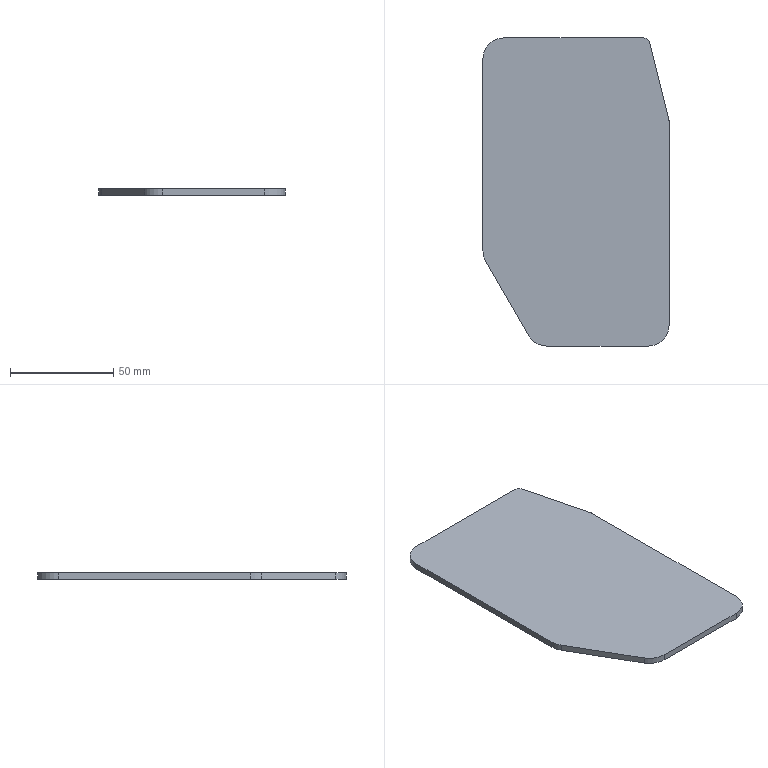Part | STEP file | Q7C1202L | 1 solid | 14 faces | box 90 x 149 x 3 mm | volume 37856 mm3 | plane 8 | cylinder 6 | commonest cylinder face diameters 20 x4 6 x2
STEP:
#1=CARTESIAN_POINT('',(0.,0.,0.));
#2=DIRECTION('',(0.,0.,1.));
#3=DIRECTION('',(1.,0.,0.));
#4=AXIS2_PLACEMENT_3D('',#1,#2,#3);
#5=CARTESIAN_POINT('',(45.,-64.5,-1.5));
#6=VERTEX_POINT('',#5);
#7=CARTESIAN_POINT('',(45.,34.131,-1.5));
#8=VERTEX_POINT('',#7);
#9=CARTESIAN_POINT('',(45.,-74.5,-1.5));
#10=DIRECTION('',(0.,1.,0.));
#11=VECTOR('',#10,1.);
#12=LINE('',#9,#11);
#13=CARTESIAN_POINT('',(45.,-74.5,1.5));
#14=DIRECTION('',(-1.,0.,0.));
#15=DIRECTION('',(0.,0.,1.));
#16=AXIS2_PLACEMENT_3D('',#13,#14,#15);
#17=PLANE('',#16);
#18=CARTESIAN_POINT('',(-3.,0.));
#19=DIRECTION('',(0.,1.));
#20=VECTOR('',#19,1.);
#21=LINE('',#18,#20);
#22=(GEOMETRIC_REPRESENTATION_CONTEXT(2)PARAMETRIC_REPRESENTATION_CONTEXT()REPRESENTATION_CONTEXT('',''));
#23=DEFINITIONAL_REPRESENTATION('',(#21),#22);
#24=PCURVE('',#17,#23);
#25=CARTESIAN_POINT('',(45.,74.5,-1.5));
#26=DIRECTION('',(0.,0.,1.));
#27=DIRECTION('',(1.,0.,0.));
#28=AXIS2_PLACEMENT_3D('',#25,#26,#27);
#29=PLANE('',#28);
#30=CARTESIAN_POINT('',(0.,-149.));
#31=DIRECTION('',(0.,1.));
#32=VECTOR('',#31,1.);
#33=LINE('',#30,#32);
#34=(GEOMETRIC_REPRESENTATION_CONTEXT(2)PARAMETRIC_REPRESENTATION_CONTEXT()REPRESENTATION_CONTEXT('',''));
#35=DEFINITIONAL_REPRESENTATION('',(#33),#34);
#36=PCURVE('',#29,#35);
#37=SURFACE_CURVE('',#12,(#24,#36),.PCURVE_S1.);
#38=EDGE_CURVE('',#6,#8,#37,.T.);
#39=ORIENTED_EDGE('',*,*,#38,.T.);
#40=CARTESIAN_POINT('',(45.,34.131,1.5));
#41=VERTEX_POINT('',#40);
#42=CARTESIAN_POINT('',(45.,34.131,1.5));
#43=DIRECTION('',(0.,0.,1.));
#44=VECTOR('',#43,1.);
#45=LINE('',#42,#44);
#46=CARTESIAN_POINT('',(0.,108.631));
#47=DIRECTION('',(1.,0.));
#48=VECTOR('',#47,1.);
#49=LINE('',#46,#48);
#50=(GEOMETRIC_REPRESENTATION_CONTEXT(2)PARAMETRIC_REPRESENTATION_CONTEXT()REPRESENTATION_CONTEXT('',''));
#51=DEFINITIONAL_REPRESENTATION('',(#49),#50);
#52=PCURVE('',#17,#51);
#53=CARTESIAN_POINT('',(42.,34.131,1.5));
#54=DIRECTION('',(0.,0.,1.));
#55=DIRECTION('',(1.,0.,0.));
#56=AXIS2_PLACEMENT_3D('',#53,#54,#55);
#57=CYLINDRICAL_SURFACE('',#56,3.);
#58=CARTESIAN_POINT('',(0.,0.));
#59=DIRECTION('',(0.,1.));
#60=VECTOR('',#59,1.);
#61=LINE('',#58,#60);
#62=(GEOMETRIC_REPRESENTATION_CONTEXT(2)PARAMETRIC_REPRESENTATION_CONTEXT()REPRESENTATION_CONTEXT('',''));
#63=DEFINITIONAL_REPRESENTATION('',(#61),#62);
#64=PCURVE('',#57,#63);
#65=SURFACE_CURVE('',#45,(#52,#64),.PCURVE_S1.);
#66=EDGE_CURVE('',#8,#41,#65,.T.);
#67=ORIENTED_EDGE('',*,*,#66,.T.);
#68=CARTESIAN_POINT('',(45.,-64.5,1.5));
#69=VERTEX_POINT('',#68);
#70=CARTESIAN_POINT('',(45.,-74.5,1.5));
#71=DIRECTION('',(0.,1.,0.));
#72=VECTOR('',#71,1.);
#73=LINE('',#70,#72);
#74=CARTESIAN_POINT('',(0.,0.));
#75=DIRECTION('',(0.,1.));
#76=VECTOR('',#75,1.);
#77=LINE('',#74,#76);
#78=(GEOMETRIC_REPRESENTATION_CONTEXT(2)PARAMETRIC_REPRESENTATION_CONTEXT()REPRESENTATION_CONTEXT('',''));
#79=DEFINITIONAL_REPRESENTATION('',(#77),#78);
#80=PCURVE('',#17,#79);
#81=CARTESIAN_POINT('',(45.,74.5,1.5));
#82=DIRECTION('',(0.,0.,1.));
#83=DIRECTION('',(1.,0.,0.));
#84=AXIS2_PLACEMENT_3D('',#81,#82,#83);
#85=PLANE('',#84);
#86=CARTESIAN_POINT('',(0.,-149.));
#87=DIRECTION('',(0.,1.));
#88=VECTOR('',#87,1.);
#89=LINE('',#86,#88);
#90=(GEOMETRIC_REPRESENTATION_CONTEXT(2)PARAMETRIC_REPRESENTATION_CONTEXT()REPRESENTATION_CONTEXT('',''));
#91=DEFINITIONAL_REPRESENTATION('',(#89),#90);
#92=PCURVE('',#85,#91);
#93=SURFACE_CURVE('',#73,(#80,#92),.PCURVE_S1.);
#94=EDGE_CURVE('',#69,#41,#93,.T.);
#95=ORIENTED_EDGE('',*,*,#94,.F.);
#96=CARTESIAN_POINT('',(45.,-64.5,1.5));
#97=DIRECTION('',(0.,0.,-1.));
#98=VECTOR('',#97,1.);
#99=LINE('',#96,#98);
#100=CARTESIAN_POINT('',(0.,10.));
#101=DIRECTION('',(-1.,0.));
#102=VECTOR('',#101,1.);
#103=LINE('',#100,#102);
#104=(GEOMETRIC_REPRESENTATION_CONTEXT(2)PARAMETRIC_REPRESENTATION_CONTEXT()REPRESENTATION_CONTEXT('',''));
#105=DEFINITIONAL_REPRESENTATION('',(#103),#104);
#106=PCURVE('',#17,#105);
#107=CARTESIAN_POINT('',(35.,-64.5,1.5));
#108=DIRECTION('',(0.,0.,-1.));
#109=DIRECTION('',(-1.,0.,0.));
#110=AXIS2_PLACEMENT_3D('',#107,#108,#109);
#111=CYLINDRICAL_SURFACE('',#110,10.);
#112=CARTESIAN_POINT('',(3.142,0.));
#113=DIRECTION('',(0.,1.));
#114=VECTOR('',#113,1.);
#115=LINE('',#112,#114);
#116=(GEOMETRIC_REPRESENTATION_CONTEXT(2)PARAMETRIC_REPRESENTATION_CONTEXT()REPRESENTATION_CONTEXT('',''));
#117=DEFINITIONAL_REPRESENTATION('',(#115),#116);
#118=PCURVE('',#111,#117);
#119=SURFACE_CURVE('',#99,(#106,#118),.PCURVE_S1.);
#120=EDGE_CURVE('',#69,#6,#119,.T.);
#121=ORIENTED_EDGE('',*,*,#120,.T.);
#122=EDGE_LOOP('',(#39,#67,#95,#121));
#123=FACE_BOUND('',#122,.T.);
#124=ADVANCED_FACE('',(#123),#17,.F.);
#125=CARTESIAN_POINT('',(32.658,74.5,1.5));
#126=VERTEX_POINT('',#125);
#127=CARTESIAN_POINT('',(-35.,74.5,1.5));
#128=VERTEX_POINT('',#127);
#129=CARTESIAN_POINT('',(45.,74.5,1.5));
#130=DIRECTION('',(-1.,0.,0.));
#131=VECTOR('',#130,1.);
#132=LINE('',#129,#131);
#133=CARTESIAN_POINT('',(45.,74.5,1.5));
#134=DIRECTION('',(0.,-1.,0.));
#135=DIRECTION('',(0.,0.,-1.));
#136=AXIS2_PLACEMENT_3D('',#133,#134,#135);
#137=PLANE('',#136);
#138=CARTESIAN_POINT('',(0.,0.));
#139=DIRECTION('',(0.,-1.));
#140=VECTOR('',#139,1.);
#141=LINE('',#138,#140);
#142=(GEOMETRIC_REPRESENTATION_CONTEXT(2)PARAMETRIC_REPRESENTATION_CONTEXT()REPRESENTATION_CONTEXT('',''));
#143=DEFINITIONAL_REPRESENTATION('',(#141),#142);
#144=PCURVE('',#137,#143);
#145=CARTESIAN_POINT('',(0.,0.));
#146=DIRECTION('',(-1.,0.));
#147=VECTOR('',#146,1.);
#148=LINE('',#145,#147);
#149=(GEOMETRIC_REPRESENTATION_CONTEXT(2)PARAMETRIC_REPRESENTATION_CONTEXT()REPRESENTATION_CONTEXT('',''));
#150=DEFINITIONAL_REPRESENTATION('',(#148),#149);
#151=PCURVE('',#85,#150);
#152=SURFACE_CURVE('',#132,(#144,#151),.PCURVE_S1.);
#153=EDGE_CURVE('',#126,#128,#152,.T.);
#154=ORIENTED_EDGE('',*,*,#153,.F.);
#155=CARTESIAN_POINT('',(32.658,74.5,-1.5));
#156=VERTEX_POINT('',#155);
#157=CARTESIAN_POINT('',(32.658,74.5,1.5));
#158=DIRECTION('',(0.,0.,-1.));
#159=VECTOR('',#158,1.);
#160=LINE('',#157,#159);
#161=CARTESIAN_POINT('',(0.,-12.342));
#162=DIRECTION('',(1.,0.));
#163=VECTOR('',#162,1.);
#164=LINE('',#161,#163);
#165=(GEOMETRIC_REPRESENTATION_CONTEXT(2)PARAMETRIC_REPRESENTATION_CONTEXT()REPRESENTATION_CONTEXT('',''));
#166=DEFINITIONAL_REPRESENTATION('',(#164),#165);
#167=PCURVE('',#137,#166);
#168=CARTESIAN_POINT('',(32.658,71.5,1.5));
#169=DIRECTION('',(0.,0.,-1.));
#170=DIRECTION('',(-1.,0.,0.));
#171=AXIS2_PLACEMENT_3D('',#168,#169,#170);
#172=CYLINDRICAL_SURFACE('',#171,3.);
#173=CARTESIAN_POINT('',(1.571,0.));
#174=DIRECTION('',(0.,1.));
#175=VECTOR('',#174,1.);
#176=LINE('',#173,#175);
#177=(GEOMETRIC_REPRESENTATION_CONTEXT(2)PARAMETRIC_REPRESENTATION_CONTEXT()REPRESENTATION_CONTEXT('',''));
#178=DEFINITIONAL_REPRESENTATION('',(#176),#177);
#179=PCURVE('',#172,#178);
#180=SURFACE_CURVE('',#160,(#167,#179),.PCURVE_S1.);
#181=EDGE_CURVE('',#126,#156,#180,.T.);
#182=ORIENTED_EDGE('',*,*,#181,.T.);
#183=CARTESIAN_POINT('',(-35.,74.5,-1.5));
#184=VERTEX_POINT('',#183);
#185=CARTESIAN_POINT('',(45.,74.5,-1.5));
#186=DIRECTION('',(-1.,0.,0.));
#187=VECTOR('',#186,1.);
#188=LINE('',#185,#187);
#189=CARTESIAN_POINT('',(3.,0.));
#190=DIRECTION('',(0.,-1.));
#191=VECTOR('',#190,1.);
#192=LINE('',#189,#191);
#193=(GEOMETRIC_REPRESENTATION_CONTEXT(2)PARAMETRIC_REPRESENTATION_CONTEXT()REPRESENTATION_CONTEXT('',''));
#194=DEFINITIONAL_REPRESENTATION('',(#192),#193);
#195=PCURVE('',#137,#194);
#196=CARTESIAN_POINT('',(0.,0.));
#197=DIRECTION('',(-1.,0.));
#198=VECTOR('',#197,1.);
#199=LINE('',#196,#198);
#200=(GEOMETRIC_REPRESENTATION_CONTEXT(2)PARAMETRIC_REPRESENTATION_CONTEXT()REPRESENTATION_CONTEXT('',''));
#201=DEFINITIONAL_REPRESENTATION('',(#199),#200);
#202=PCURVE('',#29,#201);
#203=SURFACE_CURVE('',#188,(#195,#202),.PCURVE_S1.);
#204=EDGE_CURVE('',#156,#184,#203,.T.);
#205=ORIENTED_EDGE('',*,*,#204,.T.);
#206=CARTESIAN_POINT('',(-35.,74.5,1.5));
#207=DIRECTION('',(0.,0.,1.));
#208=VECTOR('',#207,1.);
#209=LINE('',#206,#208);
#210=CARTESIAN_POINT('',(0.,-80.));
#211=DIRECTION('',(-1.,0.));
#212=VECTOR('',#211,1.);
#213=LINE('',#210,#212);
#214=(GEOMETRIC_REPRESENTATION_CONTEXT(2)PARAMETRIC_REPRESENTATION_CONTEXT()REPRESENTATION_CONTEXT('',''));
#215=DEFINITIONAL_REPRESENTATION('',(#213),#214);
#216=PCURVE('',#137,#215);
#217=CARTESIAN_POINT('',(-35.,64.5,1.5));
#218=DIRECTION('',(0.,0.,-1.));
#219=DIRECTION('',(-1.,0.,0.));
#220=AXIS2_PLACEMENT_3D('',#217,#218,#219);
#221=CYLINDRICAL_SURFACE('',#220,10.);
#222=CARTESIAN_POINT('',(1.571,0.));
#223=DIRECTION('',(0.,-1.));
#224=VECTOR('',#223,1.);
#225=LINE('',#222,#224);
#226=(GEOMETRIC_REPRESENTATION_CONTEXT(2)PARAMETRIC_REPRESENTATION_CONTEXT()REPRESENTATION_CONTEXT('',''));
#227=DEFINITIONAL_REPRESENTATION('',(#225),#226);
#228=PCURVE('',#221,#227);
#229=SURFACE_CURVE('',#209,(#216,#228),.PCURVE_S1.);
#230=EDGE_CURVE('',#184,#128,#229,.T.);
#231=ORIENTED_EDGE('',*,*,#230,.T.);
#232=EDGE_LOOP('',(#154,#182,#205,#231));
#233=FACE_BOUND('',#232,.T.);
#234=ADVANCED_FACE('',(#233),#137,.F.);
#235=CARTESIAN_POINT('',(-45.,64.5,-1.5));
#236=VERTEX_POINT('',#235);
#237=CARTESIAN_POINT('',(-45.,-28.519,-1.5));
#238=VERTEX_POINT('',#237);
#239=CARTESIAN_POINT('',(-45.,74.5,-1.5));
#240=DIRECTION('',(0.,-1.,0.));
#241=VECTOR('',#240,1.);
#242=LINE('',#239,#241);
#243=CARTESIAN_POINT('',(-45.,74.5,1.5));
#244=DIRECTION('',(1.,0.,0.));
#245=DIRECTION('',(0.,1.,0.));
#246=AXIS2_PLACEMENT_3D('',#243,#244,#245);
#247=PLANE('',#246);
#248=CARTESIAN_POINT('',(0.,-3.));
#249=DIRECTION('',(-1.,0.));
#250=VECTOR('',#249,1.);
#251=LINE('',#248,#250);
#252=(GEOMETRIC_REPRESENTATION_CONTEXT(2)PARAMETRIC_REPRESENTATION_CONTEXT()REPRESENTATION_CONTEXT('',''));
#253=DEFINITIONAL_REPRESENTATION('',(#251),#252);
#254=PCURVE('',#247,#253);
#255=CARTESIAN_POINT('',(-90.,0.));
#256=DIRECTION('',(0.,-1.));
#257=VECTOR('',#256,1.);
#258=LINE('',#255,#257);
#259=(GEOMETRIC_REPRESENTATION_CONTEXT(2)PARAMETRIC_REPRESENTATION_CONTEXT()REPRESENTATION_CONTEXT('',''));
#260=DEFINITIONAL_REPRESENTATION('',(#258),#259);
#261=PCURVE('',#29,#260);
#262=SURFACE_CURVE('',#242,(#254,#261),.PCURVE_S1.);
#263=EDGE_CURVE('',#236,#238,#262,.T.);
#264=ORIENTED_EDGE('',*,*,#263,.T.);
#265=CARTESIAN_POINT('',(-45.,-28.519,1.5));
#266=VERTEX_POINT('',#265);
#267=CARTESIAN_POINT('',(-45.,-28.519,1.5));
#268=DIRECTION('',(0.,0.,1.));
#269=VECTOR('',#268,1.);
#270=LINE('',#267,#269);
#271=CARTESIAN_POINT('',(-103.019,0.));
#272=DIRECTION('',(0.,1.));
#273=VECTOR('',#272,1.);
#274=LINE('',#271,#273);
#275=(GEOMETRIC_REPRESENTATION_CONTEXT(2)PARAMETRIC_REPRESENTATION_CONTEXT()REPRESENTATION_CONTEXT('',''));
#276=DEFINITIONAL_REPRESENTATION('',(#274),#275);
#277=PCURVE('',#247,#276);
#278=CARTESIAN_POINT('',(-35.,-28.519,1.5));
#279=DIRECTION('',(0.,0.,-1.));
#280=DIRECTION('',(-1.,0.,0.));
#281=AXIS2_PLACEMENT_3D('',#278,#279,#280);
#282=CYLINDRICAL_SURFACE('',#281,10.);
#283=CARTESIAN_POINT('',(6.283,0.));
#284=DIRECTION('',(0.,-1.));
#285=VECTOR('',#284,1.);
#286=LINE('',#283,#285);
#287=(GEOMETRIC_REPRESENTATION_CONTEXT(2)PARAMETRIC_REPRESENTATION_CONTEXT()REPRESENTATION_CONTEXT('',''));
#288=DEFINITIONAL_REPRESENTATION('',(#286),#287);
#289=PCURVE('',#282,#288);
#290=SURFACE_CURVE('',#270,(#277,#289),.PCURVE_S1.);
#291=EDGE_CURVE('',#238,#266,#290,.T.);
#292=ORIENTED_EDGE('',*,*,#291,.T.);
#293=CARTESIAN_POINT('',(-45.,64.5,1.5));
#294=VERTEX_POINT('',#293);
#295=CARTESIAN_POINT('',(-45.,74.5,1.5));
#296=DIRECTION('',(0.,-1.,0.));
#297=VECTOR('',#296,1.);
#298=LINE('',#295,#297);
#299=CARTESIAN_POINT('',(0.,0.));
#300=DIRECTION('',(-1.,0.));
#301=VECTOR('',#300,1.);
#302=LINE('',#299,#301);
#303=(GEOMETRIC_REPRESENTATION_CONTEXT(2)PARAMETRIC_REPRESENTATION_CONTEXT()REPRESENTATION_CONTEXT('',''));
#304=DEFINITIONAL_REPRESENTATION('',(#302),#303);
#305=PCURVE('',#247,#304);
#306=CARTESIAN_POINT('',(-90.,0.));
#307=DIRECTION('',(0.,-1.));
#308=VECTOR('',#307,1.);
#309=LINE('',#306,#308);
#310=(GEOMETRIC_REPRESENTATION_CONTEXT(2)PARAMETRIC_REPRESENTATION_CONTEXT()REPRESENTATION_CONTEXT('',''));
#311=DEFINITIONAL_REPRESENTATION('',(#309),#310);
#312=PCURVE('',#85,#311);
#313=SURFACE_CURVE('',#298,(#305,#312),.PCURVE_S1.);
#314=EDGE_CURVE('',#294,#266,#313,.T.);
#315=ORIENTED_EDGE('',*,*,#314,.F.);
#316=CARTESIAN_POINT('',(-45.,64.5,1.5));
#317=DIRECTION('',(0.,0.,-1.));
#318=VECTOR('',#317,1.);
#319=LINE('',#316,#318);
#320=CARTESIAN_POINT('',(-10.,0.));
#321=DIRECTION('',(0.,-1.));
#322=VECTOR('',#321,1.);
#323=LINE('',#320,#322);
#324=(GEOMETRIC_REPRESENTATION_CONTEXT(2)PARAMETRIC_REPRESENTATION_CONTEXT()REPRESENTATION_CONTEXT('',''));
#325=DEFINITIONAL_REPRESENTATION('',(#323),#324);
#326=PCURVE('',#247,#325);
#327=CARTESIAN_POINT('',(0.,0.));
#328=DIRECTION('',(0.,1.));
#329=VECTOR('',#328,1.);
#330=LINE('',#327,#329);
#331=(GEOMETRIC_REPRESENTATION_CONTEXT(2)PARAMETRIC_REPRESENTATION_CONTEXT()REPRESENTATION_CONTEXT('',''));
#332=DEFINITIONAL_REPRESENTATION('',(#330),#331);
#333=PCURVE('',#221,#332);
#334=SURFACE_CURVE('',#319,(#326,#333),.PCURVE_S1.);
#335=EDGE_CURVE('',#294,#236,#334,.T.);
#336=ORIENTED_EDGE('',*,*,#335,.T.);
#337=EDGE_LOOP('',(#264,#292,#315,#336));
#338=FACE_BOUND('',#337,.T.);
#339=ADVANCED_FACE('',(#338),#247,.F.);
#340=CARTESIAN_POINT('',(-43.66,-33.519,1.5));
#341=VERTEX_POINT('',#340);
#342=CARTESIAN_POINT('',(-22.887,-69.5,1.5));
#343=VERTEX_POINT('',#342);
#344=CARTESIAN_POINT('',(-45.,-31.199,1.5));
#345=DIRECTION('',(0.5,-0.866,0.));
#346=VECTOR('',#345,1.);
#347=LINE('',#344,#346);
#348=CARTESIAN_POINT('',(-45.,-31.199,1.5));
#349=DIRECTION('',(0.866,0.5,0.));
#350=DIRECTION('',(-0.5,0.866,0.));
#351=AXIS2_PLACEMENT_3D('',#348,#349,#350);
#352=PLANE('',#351);
#353=CARTESIAN_POINT('',(0.,0.));
#354=DIRECTION('',(-1.,0.));
#355=VECTOR('',#354,1.);
#356=LINE('',#353,#355);
#357=(GEOMETRIC_REPRESENTATION_CONTEXT(2)PARAMETRIC_REPRESENTATION_CONTEXT()REPRESENTATION_CONTEXT('',''));
#358=DEFINITIONAL_REPRESENTATION('',(#356),#357);
#359=PCURVE('',#352,#358);
#360=CARTESIAN_POINT('',(-90.,-105.699));
#361=DIRECTION('',(0.5,-0.866));
#362=VECTOR('',#361,1.);
#363=LINE('',#360,#362);
#364=(GEOMETRIC_REPRESENTATION_CONTEXT(2)PARAMETRIC_REPRESENTATION_CONTEXT()REPRESENTATION_CONTEXT('',''));
#365=DEFINITIONAL_REPRESENTATION('',(#363),#364);
#366=PCURVE('',#85,#365);
#367=SURFACE_CURVE('',#347,(#359,#366),.PCURVE_S1.);
#368=EDGE_CURVE('',#341,#343,#367,.T.);
#369=ORIENTED_EDGE('',*,*,#368,.F.);
#370=CARTESIAN_POINT('',(-43.66,-33.519,-1.5));
#371=VERTEX_POINT('',#370);
#372=CARTESIAN_POINT('',(-43.66,-33.519,1.5));
#373=DIRECTION('',(0.,0.,-1.));
#374=VECTOR('',#373,1.);
#375=LINE('',#372,#374);
#376=CARTESIAN_POINT('',(-2.679,0.));
#377=DIRECTION('',(0.,-1.));
#378=VECTOR('',#377,1.);
#379=LINE('',#376,#378);
#380=(GEOMETRIC_REPRESENTATION_CONTEXT(2)PARAMETRIC_REPRESENTATION_CONTEXT()REPRESENTATION_CONTEXT('',''));
#381=DEFINITIONAL_REPRESENTATION('',(#379),#380);
#382=PCURVE('',#352,#381);
#383=CARTESIAN_POINT('',(5.76,0.));
#384=DIRECTION('',(0.,1.));
#385=VECTOR('',#384,1.);
#386=LINE('',#383,#385);
#387=(GEOMETRIC_REPRESENTATION_CONTEXT(2)PARAMETRIC_REPRESENTATION_CONTEXT()REPRESENTATION_CONTEXT('',''));
#388=DEFINITIONAL_REPRESENTATION('',(#386),#387);
#389=PCURVE('',#282,#388);
#390=SURFACE_CURVE('',#375,(#382,#389),.PCURVE_S1.);
#391=EDGE_CURVE('',#341,#371,#390,.T.);
#392=ORIENTED_EDGE('',*,*,#391,.T.);
#393=CARTESIAN_POINT('',(-22.887,-69.5,-1.5));
#394=VERTEX_POINT('',#393);
#395=CARTESIAN_POINT('',(-45.,-31.199,-1.5));
#396=DIRECTION('',(0.5,-0.866,0.));
#397=VECTOR('',#396,1.);
#398=LINE('',#395,#397);
#399=CARTESIAN_POINT('',(0.,-3.));
#400=DIRECTION('',(-1.,0.));
#401=VECTOR('',#400,1.);
#402=LINE('',#399,#401);
#403=(GEOMETRIC_REPRESENTATION_CONTEXT(2)PARAMETRIC_REPRESENTATION_CONTEXT()REPRESENTATION_CONTEXT('',''));
#404=DEFINITIONAL_REPRESENTATION('',(#402),#403);
#405=PCURVE('',#352,#404);
#406=CARTESIAN_POINT('',(-90.,-105.699));
#407=DIRECTION('',(0.5,-0.866));
#408=VECTOR('',#407,1.);
#409=LINE('',#406,#408);
#410=(GEOMETRIC_REPRESENTATION_CONTEXT(2)PARAMETRIC_REPRESENTATION_CONTEXT()REPRESENTATION_CONTEXT('',''));
#411=DEFINITIONAL_REPRESENTATION('',(#409),#410);
#412=PCURVE('',#29,#411);
#413=SURFACE_CURVE('',#398,(#405,#412),.PCURVE_S1.);
#414=EDGE_CURVE('',#371,#394,#413,.T.);
#415=ORIENTED_EDGE('',*,*,#414,.T.);
#416=CARTESIAN_POINT('',(-22.887,-69.5,1.5));
#417=DIRECTION('',(0.,0.,1.));
#418=VECTOR('',#417,1.);
#419=LINE('',#416,#418);
#420=CARTESIAN_POINT('',(-44.226,0.));
#421=DIRECTION('',(0.,1.));
#422=VECTOR('',#421,1.);
#423=LINE('',#420,#422);
#424=(GEOMETRIC_REPRESENTATION_CONTEXT(2)PARAMETRIC_REPRESENTATION_CONTEXT()REPRESENTATION_CONTEXT('',''));
#425=DEFINITIONAL_REPRESENTATION('',(#423),#424);
#426=PCURVE('',#352,#425);
#427=CARTESIAN_POINT('',(-14.226,-64.5,1.5));
#428=DIRECTION('',(0.,0.,-1.));
#429=DIRECTION('',(-1.,0.,0.));
#430=AXIS2_PLACEMENT_3D('',#427,#428,#429);
#431=CYLINDRICAL_SURFACE('',#430,10.);
#432=CARTESIAN_POINT('',(5.76,0.));
#433=DIRECTION('',(0.,-1.));
#434=VECTOR('',#433,1.);
#435=LINE('',#432,#434);
#436=(GEOMETRIC_REPRESENTATION_CONTEXT(2)PARAMETRIC_REPRESENTATION_CONTEXT()REPRESENTATION_CONTEXT('',''));
#437=DEFINITIONAL_REPRESENTATION('',(#435),#436);
#438=PCURVE('',#431,#437);
#439=SURFACE_CURVE('',#419,(#426,#438),.PCURVE_S1.);
#440=EDGE_CURVE('',#394,#343,#439,.T.);
#441=ORIENTED_EDGE('',*,*,#440,.T.);
#442=EDGE_LOOP('',(#369,#392,#415,#441));
#443=FACE_BOUND('',#442,.T.);
#444=ADVANCED_FACE('',(#443),#352,.F.);
#445=CARTESIAN_POINT('',(-14.226,-74.5,1.5));
#446=VERTEX_POINT('',#445);
#447=CARTESIAN_POINT('',(35.,-74.5,1.5));
#448=VERTEX_POINT('',#447);
#449=CARTESIAN_POINT('',(-20.,-74.5,1.5));
#450=DIRECTION('',(1.,0.,0.));
#451=VECTOR('',#450,1.);
#452=LINE('',#449,#451);
#453=CARTESIAN_POINT('',(-20.,-74.5,1.5));
#454=DIRECTION('',(0.,1.,0.));
#455=DIRECTION('',(0.,0.,1.));
#456=AXIS2_PLACEMENT_3D('',#453,#454,#455);
#457=PLANE('',#456);
#458=CARTESIAN_POINT('',(0.,0.));
#459=DIRECTION('',(0.,1.));
#460=VECTOR('',#459,1.);
#461=LINE('',#458,#460);
#462=(GEOMETRIC_REPRESENTATION_CONTEXT(2)PARAMETRIC_REPRESENTATION_CONTEXT()REPRESENTATION_CONTEXT('',''));
#463=DEFINITIONAL_REPRESENTATION('',(#461),#462);
#464=PCURVE('',#457,#463);
#465=CARTESIAN_POINT('',(-65.,-149.));
#466=DIRECTION('',(1.,0.));
#467=VECTOR('',#466,1.);
#468=LINE('',#465,#467);
#469=(GEOMETRIC_REPRESENTATION_CONTEXT(2)PARAMETRIC_REPRESENTATION_CONTEXT()REPRESENTATION_CONTEXT('',''));
#470=DEFINITIONAL_REPRESENTATION('',(#468),#469);
#471=PCURVE('',#85,#470);
#472=SURFACE_CURVE('',#452,(#464,#471),.PCURVE_S1.);
#473=EDGE_CURVE('',#446,#448,#472,.T.);
#474=ORIENTED_EDGE('',*,*,#473,.F.);
#475=CARTESIAN_POINT('',(-14.226,-74.5,-1.5));
#476=VERTEX_POINT('',#475);
#477=CARTESIAN_POINT('',(-14.226,-74.5,1.5));
#478=DIRECTION('',(0.,0.,-1.));
#479=VECTOR('',#478,1.);
#480=LINE('',#477,#479);
#481=CARTESIAN_POINT('',(0.,5.774));
#482=DIRECTION('',(-1.,0.));
#483=VECTOR('',#482,1.);
#484=LINE('',#481,#483);
#485=(GEOMETRIC_REPRESENTATION_CONTEXT(2)PARAMETRIC_REPRESENTATION_CONTEXT()REPRESENTATION_CONTEXT('',''));
#486=DEFINITIONAL_REPRESENTATION('',(#484),#485);
#487=PCURVE('',#457,#486);
#488=CARTESIAN_POINT('',(4.712,0.));
#489=DIRECTION('',(0.,1.));
#490=VECTOR('',#489,1.);
#491=LINE('',#488,#490);
#492=(GEOMETRIC_REPRESENTATION_CONTEXT(2)PARAMETRIC_REPRESENTATION_CONTEXT()REPRESENTATION_CONTEXT('',''));
#493=DEFINITIONAL_REPRESENTATION('',(#491),#492);
#494=PCURVE('',#431,#493);
#495=SURFACE_CURVE('',#480,(#487,#494),.PCURVE_S1.);
#496=EDGE_CURVE('',#446,#476,#495,.T.);
#497=ORIENTED_EDGE('',*,*,#496,.T.);
#498=CARTESIAN_POINT('',(35.,-74.5,-1.5));
#499=VERTEX_POINT('',#498);
#500=CARTESIAN_POINT('',(-20.,-74.5,-1.5));
#501=DIRECTION('',(1.,0.,0.));
#502=VECTOR('',#501,1.);
#503=LINE('',#500,#502);
#504=CARTESIAN_POINT('',(-3.,0.));
#505=DIRECTION('',(0.,1.));
#506=VECTOR('',#505,1.);
#507=LINE('',#504,#506);
#508=(GEOMETRIC_REPRESENTATION_CONTEXT(2)PARAMETRIC_REPRESENTATION_CONTEXT()REPRESENTATION_CONTEXT('',''));
#509=DEFINITIONAL_REPRESENTATION('',(#507),#508);
#510=PCURVE('',#457,#509);
#511=CARTESIAN_POINT('',(-65.,-149.));
#512=DIRECTION('',(1.,0.));
#513=VECTOR('',#512,1.);
#514=LINE('',#511,#513);
#515=(GEOMETRIC_REPRESENTATION_CONTEXT(2)PARAMETRIC_REPRESENTATION_CONTEXT()REPRESENTATION_CONTEXT('',''));
#516=DEFINITIONAL_REPRESENTATION('',(#514),#515);
#517=PCURVE('',#29,#516);
#518=SURFACE_CURVE('',#503,(#510,#517),.PCURVE_S1.);
#519=EDGE_CURVE('',#476,#499,#518,.T.);
#520=ORIENTED_EDGE('',*,*,#519,.T.);
#521=CARTESIAN_POINT('',(35.,-74.5,1.5));
#522=DIRECTION('',(0.,0.,1.));
#523=VECTOR('',#522,1.);
#524=LINE('',#521,#523);
#525=CARTESIAN_POINT('',(0.,55.));
#526=DIRECTION('',(1.,0.));
#527=VECTOR('',#526,1.);
#528=LINE('',#525,#527);
#529=(GEOMETRIC_REPRESENTATION_CONTEXT(2)PARAMETRIC_REPRESENTATION_CONTEXT()REPRESENTATION_CONTEXT('',''));
#530=DEFINITIONAL_REPRESENTATION('',(#528),#529);
#531=PCURVE('',#457,#530);
#532=CARTESIAN_POINT('',(4.712,0.));
#533=DIRECTION('',(0.,-1.));
#534=VECTOR('',#533,1.);
#535=LINE('',#532,#534);
#536=(GEOMETRIC_REPRESENTATION_CONTEXT(2)PARAMETRIC_REPRESENTATION_CONTEXT()REPRESENTATION_CONTEXT('',''));
#537=DEFINITIONAL_REPRESENTATION('',(#535),#536);
#538=PCURVE('',#111,#537);
#539=SURFACE_CURVE('',#524,(#531,#538),.PCURVE_S1.);
#540=EDGE_CURVE('',#499,#448,#539,.T.);
#541=ORIENTED_EDGE('',*,*,#540,.T.);
#542=EDGE_LOOP('',(#474,#497,#520,#541));
#543=FACE_BOUND('',#542,.T.);
#544=ADVANCED_FACE('',(#543),#457,.F.);
#545=ORIENTED_EDGE('',*,*,#94,.T.);
#546=CARTESIAN_POINT('',(44.91,34.858,1.5));
#547=VERTEX_POINT('',#546);
#548=CARTESIAN_POINT('',(42.,34.131,1.5));
#549=DIRECTION('',(0.,0.,1.));
#550=DIRECTION('',(1.,0.,0.));
#551=AXIS2_PLACEMENT_3D('',#548,#549,#550);
#552=CIRCLE('',#551,3.);
#553=CARTESIAN_POINT('',(-3.,-40.369));
#554=DIRECTION('',(1.,0.));
#555=AXIS2_PLACEMENT_2D('',#553,#554);
#556=CIRCLE('',#555,3.);
#557=(GEOMETRIC_REPRESENTATION_CONTEXT(2)PARAMETRIC_REPRESENTATION_CONTEXT()REPRESENTATION_CONTEXT('',''));
#558=DEFINITIONAL_REPRESENTATION('',(#556),#557);
#559=PCURVE('',#85,#558);
#560=CARTESIAN_POINT('',(0.,0.));
#561=DIRECTION('',(1.,0.));
#562=VECTOR('',#561,1.);
#563=LINE('',#560,#562);
#564=(GEOMETRIC_REPRESENTATION_CONTEXT(2)PARAMETRIC_REPRESENTATION_CONTEXT()REPRESENTATION_CONTEXT('',''));
#565=DEFINITIONAL_REPRESENTATION('',(#563),#564);
#566=PCURVE('',#57,#565);
#567=SURFACE_CURVE('',#552,(#559,#566),.PCURVE_S1.);
#568=EDGE_CURVE('',#41,#547,#567,.T.);
#569=ORIENTED_EDGE('',*,*,#568,.T.);
#570=CARTESIAN_POINT('',(35.568,72.228,1.5));
#571=VERTEX_POINT('',#570);
#572=CARTESIAN_POINT('',(35.,74.5,1.5));
#573=DIRECTION('',(0.2425,-0.9701,0.));
#574=VECTOR('',#573,1.);
#575=LINE('',#572,#574);
#576=CARTESIAN_POINT('',(-10.,0.));
#577=DIRECTION('',(0.2425,-0.9701));
#578=VECTOR('',#577,1.);
#579=LINE('',#576,#578);
#580=(GEOMETRIC_REPRESENTATION_CONTEXT(2)PARAMETRIC_REPRESENTATION_CONTEXT()REPRESENTATION_CONTEXT('',''));
#581=DEFINITIONAL_REPRESENTATION('',(#579),#580);
#582=PCURVE('',#85,#581);
#583=CARTESIAN_POINT('',(35.,74.5,-8.5));
#584=DIRECTION('',(-0.9701,-0.2425,0.));
#585=DIRECTION('',(0.2425,-0.9701,0.));
#586=AXIS2_PLACEMENT_3D('',#583,#584,#585);
#587=PLANE('',#586);
#588=CARTESIAN_POINT('',(0.,10.));
#589=DIRECTION('',(1.,0.));
#590=VECTOR('',#589,1.);
#591=LINE('',#588,#590);
#592=(GEOMETRIC_REPRESENTATION_CONTEXT(2)PARAMETRIC_REPRESENTATION_CONTEXT()REPRESENTATION_CONTEXT('',''));
#593=DEFINITIONAL_REPRESENTATION('',(#591),#592);
#594=PCURVE('',#587,#593);
#595=SURFACE_CURVE('',#575,(#582,#594),.PCURVE_S1.);
#596=EDGE_CURVE('',#571,#547,#595,.T.);
#597=ORIENTED_EDGE('',*,*,#596,.F.);
#598=CARTESIAN_POINT('',(32.658,71.5,1.5));
#599=DIRECTION('',(0.,0.,1.));
#600=DIRECTION('',(1.,0.,0.));
#601=AXIS2_PLACEMENT_3D('',#598,#599,#600);
#602=CIRCLE('',#601,3.);
#603=CARTESIAN_POINT('',(-12.342,-3.));
#604=DIRECTION('',(1.,0.));
#605=AXIS2_PLACEMENT_2D('',#603,#604);
#606=CIRCLE('',#605,3.);
#607=(GEOMETRIC_REPRESENTATION_CONTEXT(2)PARAMETRIC_REPRESENTATION_CONTEXT()REPRESENTATION_CONTEXT('',''));
#608=DEFINITIONAL_REPRESENTATION('',(#606),#607);
#609=PCURVE('',#85,#608);
#610=CARTESIAN_POINT('',(3.142,0.));
#611=DIRECTION('',(-1.,0.));
#612=VECTOR('',#611,1.);
#613=LINE('',#610,#612);
#614=(GEOMETRIC_REPRESENTATION_CONTEXT(2)PARAMETRIC_REPRESENTATION_CONTEXT()REPRESENTATION_CONTEXT('',''));
#615=DEFINITIONAL_REPRESENTATION('',(#613),#614);
#616=PCURVE('',#172,#615);
#617=SURFACE_CURVE('',#602,(#609,#616),.PCURVE_S1.);
#618=EDGE_CURVE('',#571,#126,#617,.T.);
#619=ORIENTED_EDGE('',*,*,#618,.T.);
#620=ORIENTED_EDGE('',*,*,#153,.T.);
#621=CARTESIAN_POINT('',(-35.,64.5,1.5));
#622=DIRECTION('',(0.,0.,1.));
#623=DIRECTION('',(1.,0.,0.));
#624=AXIS2_PLACEMENT_3D('',#621,#622,#623);
#625=CIRCLE('',#624,10.);
#626=CARTESIAN_POINT('',(-80.,-10.));
#627=DIRECTION('',(1.,0.));
#628=AXIS2_PLACEMENT_2D('',#626,#627);
#629=CIRCLE('',#628,10.);
#630=(GEOMETRIC_REPRESENTATION_CONTEXT(2)PARAMETRIC_REPRESENTATION_CONTEXT()REPRESENTATION_CONTEXT('',''));
#631=DEFINITIONAL_REPRESENTATION('',(#629),#630);
#632=PCURVE('',#85,#631);
#633=CARTESIAN_POINT('',(3.142,0.));
#634=DIRECTION('',(-1.,0.));
#635=VECTOR('',#634,1.);
#636=LINE('',#633,#635);
#637=(GEOMETRIC_REPRESENTATION_CONTEXT(2)PARAMETRIC_REPRESENTATION_CONTEXT()REPRESENTATION_CONTEXT('',''));
#638=DEFINITIONAL_REPRESENTATION('',(#636),#637);
#639=PCURVE('',#221,#638);
#640=SURFACE_CURVE('',#625,(#632,#639),.PCURVE_S1.);
#641=EDGE_CURVE('',#128,#294,#640,.T.);
#642=ORIENTED_EDGE('',*,*,#641,.T.);
#643=ORIENTED_EDGE('',*,*,#314,.T.);
#644=CARTESIAN_POINT('',(-35.,-28.519,1.5));
#645=DIRECTION('',(0.,0.,1.));
#646=DIRECTION('',(1.,0.,0.));
#647=AXIS2_PLACEMENT_3D('',#644,#645,#646);
#648=CIRCLE('',#647,10.);
#649=CARTESIAN_POINT('',(-80.,-103.019));
#650=DIRECTION('',(1.,0.));
#651=AXIS2_PLACEMENT_2D('',#649,#650);
#652=CIRCLE('',#651,10.);
#653=(GEOMETRIC_REPRESENTATION_CONTEXT(2)PARAMETRIC_REPRESENTATION_CONTEXT()REPRESENTATION_CONTEXT('',''));
#654=DEFINITIONAL_REPRESENTATION('',(#652),#653);
#655=PCURVE('',#85,#654);
#656=CARTESIAN_POINT('',(9.425,0.));
#657=DIRECTION('',(-1.,0.));
#658=VECTOR('',#657,1.);
#659=LINE('',#656,#658);
#660=(GEOMETRIC_REPRESENTATION_CONTEXT(2)PARAMETRIC_REPRESENTATION_CONTEXT()REPRESENTATION_CONTEXT('',''));
#661=DEFINITIONAL_REPRESENTATION('',(#659),#660);
#662=PCURVE('',#282,#661);
#663=SURFACE_CURVE('',#648,(#655,#662),.PCURVE_S1.);
#664=EDGE_CURVE('',#266,#341,#663,.T.);
#665=ORIENTED_EDGE('',*,*,#664,.T.);
#666=ORIENTED_EDGE('',*,*,#368,.T.);
#667=CARTESIAN_POINT('',(-14.226,-64.5,1.5));
#668=DIRECTION('',(0.,0.,1.));
#669=DIRECTION('',(1.,0.,0.));
#670=AXIS2_PLACEMENT_3D('',#667,#668,#669);
#671=CIRCLE('',#670,10.);
#672=CARTESIAN_POINT('',(-59.226,-139.));
#673=DIRECTION('',(1.,0.));
#674=AXIS2_PLACEMENT_2D('',#672,#673);
#675=CIRCLE('',#674,10.);
#676=(GEOMETRIC_REPRESENTATION_CONTEXT(2)PARAMETRIC_REPRESENTATION_CONTEXT()REPRESENTATION_CONTEXT('',''));
#677=DEFINITIONAL_REPRESENTATION('',(#675),#676);
#678=PCURVE('',#85,#677);
#679=CARTESIAN_POINT('',(9.425,0.));
#680=DIRECTION('',(-1.,0.));
#681=VECTOR('',#680,1.);
#682=LINE('',#679,#681);
#683=(GEOMETRIC_REPRESENTATION_CONTEXT(2)PARAMETRIC_REPRESENTATION_CONTEXT()REPRESENTATION_CONTEXT('',''));
#684=DEFINITIONAL_REPRESENTATION('',(#682),#683);
#685=PCURVE('',#431,#684);
#686=SURFACE_CURVE('',#671,(#678,#685),.PCURVE_S1.);
#687=EDGE_CURVE('',#343,#446,#686,.T.);
#688=ORIENTED_EDGE('',*,*,#687,.T.);
#689=ORIENTED_EDGE('',*,*,#473,.T.);
#690=CARTESIAN_POINT('',(35.,-64.5,1.5));
#691=DIRECTION('',(0.,0.,1.));
#692=DIRECTION('',(1.,0.,0.));
#693=AXIS2_PLACEMENT_3D('',#690,#691,#692);
#694=CIRCLE('',#693,10.);
#695=CARTESIAN_POINT('',(-10.,-139.));
#696=DIRECTION('',(1.,0.));
#697=AXIS2_PLACEMENT_2D('',#695,#696);
#698=CIRCLE('',#697,10.);
#699=(GEOMETRIC_REPRESENTATION_CONTEXT(2)PARAMETRIC_REPRESENTATION_CONTEXT()REPRESENTATION_CONTEXT('',''));
#700=DEFINITIONAL_REPRESENTATION('',(#698),#699);
#701=PCURVE('',#85,#700);
#702=CARTESIAN_POINT('',(9.425,0.));
#703=DIRECTION('',(-1.,0.));
#704=VECTOR('',#703,1.);
#705=LINE('',#702,#704);
#706=(GEOMETRIC_REPRESENTATION_CONTEXT(2)PARAMETRIC_REPRESENTATION_CONTEXT()REPRESENTATION_CONTEXT('',''));
#707=DEFINITIONAL_REPRESENTATION('',(#705),#706);
#708=PCURVE('',#111,#707);
#709=SURFACE_CURVE('',#694,(#701,#708),.PCURVE_S1.);
#710=EDGE_CURVE('',#448,#69,#709,.T.);
#711=ORIENTED_EDGE('',*,*,#710,.T.);
#712=EDGE_LOOP('',(#545,#569,#597,#619,#620,#642,#643,#665,#666,#688,#689,#711));
#713=FACE_BOUND('',#712,.T.);
#714=ADVANCED_FACE('',(#713),#85,.T.);
#715=CARTESIAN_POINT('',(35.568,72.228,-1.5));
#716=VERTEX_POINT('',#715);
#717=CARTESIAN_POINT('',(44.91,34.858,-1.5));
#718=VERTEX_POINT('',#717);
#719=CARTESIAN_POINT('',(35.588,72.147,-1.5));
#720=DIRECTION('',(0.2425,-0.9701,0.));
#721=VECTOR('',#720,1.);
#722=LINE('',#719,#721);
#723=CARTESIAN_POINT('',(-9.412,-2.353));
#724=DIRECTION('',(0.2425,-0.9701));
#725=VECTOR('',#724,1.);
#726=LINE('',#723,#725);
#727=(GEOMETRIC_REPRESENTATION_CONTEXT(2)PARAMETRIC_REPRESENTATION_CONTEXT()REPRESENTATION_CONTEXT('',''));
#728=DEFINITIONAL_REPRESENTATION('',(#726),#727);
#729=PCURVE('',#29,#728);
#730=CARTESIAN_POINT('',(2.425,7.));
#731=DIRECTION('',(1.,0.));
#732=VECTOR('',#731,1.);
#733=LINE('',#730,#732);
#734=(GEOMETRIC_REPRESENTATION_CONTEXT(2)PARAMETRIC_REPRESENTATION_CONTEXT()REPRESENTATION_CONTEXT('',''));
#735=DEFINITIONAL_REPRESENTATION('',(#733),#734);
#736=PCURVE('',#587,#735);
#737=SURFACE_CURVE('',#722,(#729,#736),.PCURVE_S1.);
#738=EDGE_CURVE('',#716,#718,#737,.T.);
#739=ORIENTED_EDGE('',*,*,#738,.T.);
#740=CARTESIAN_POINT('',(42.,34.131,-1.5));
#741=DIRECTION('',(0.,0.,-1.));
#742=DIRECTION('',(1.,0.,0.));
#743=AXIS2_PLACEMENT_3D('',#740,#741,#742);
#744=CIRCLE('',#743,3.);
#745=CARTESIAN_POINT('',(0.,-40.369));
#746=CARTESIAN_POINT('',(0.,-45.565));
#747=CARTESIAN_POINT('',(-4.5,-42.967));
#748=CARTESIAN_POINT('',(-9.,-40.369));
#749=CARTESIAN_POINT('',(-4.5,-37.771));
#750=CARTESIAN_POINT('',(0.,-35.173));
#751=CARTESIAN_POINT('',(0.,-40.369));
#752=(BOUNDED_CURVE()B_SPLINE_CURVE(2,(#745,#746,#747,#748,#749,#750,#751),.UNSPECIFIED.,.T.,.F.)B_SPLINE_CURVE_WITH_KNOTS((1,2,2,2,2,1),(-2.094,0.,2.094,4.189,6.283,8.378),.UNSPECIFIED.)CURVE()GEOMETRIC_REPRESENTATION_ITEM()RATIONAL_B_SPLINE_CURVE((1.,0.5,1.,0.5,1.,0.5,1.))REPRESENTATION_ITEM(''));
#753=(GEOMETRIC_REPRESENTATION_CONTEXT(2)PARAMETRIC_REPRESENTATION_CONTEXT()REPRESENTATION_CONTEXT('',''));
#754=DEFINITIONAL_REPRESENTATION('',(#752),#753);
#755=PCURVE('',#29,#754);
#756=CARTESIAN_POINT('',(6.283,-3.));
#757=DIRECTION('',(-1.,0.));
#758=VECTOR('',#757,1.);
#759=LINE('',#756,#758);
#760=(GEOMETRIC_REPRESENTATION_CONTEXT(2)PARAMETRIC_REPRESENTATION_CONTEXT()REPRESENTATION_CONTEXT('',''));
#761=DEFINITIONAL_REPRESENTATION('',(#759),#760);
#762=PCURVE('',#57,#761);
#763=SURFACE_CURVE('',#744,(#755,#762),.PCURVE_S1.);
#764=EDGE_CURVE('',#718,#8,#763,.T.);
#765=ORIENTED_EDGE('',*,*,#764,.T.);
#766=ORIENTED_EDGE('',*,*,#38,.F.);
#767=CARTESIAN_POINT('',(35.,-64.5,-1.5));
#768=DIRECTION('',(0.,0.,-1.));
#769=DIRECTION('',(1.,0.,0.));
#770=AXIS2_PLACEMENT_3D('',#767,#768,#769);
#771=CIRCLE('',#770,10.);
#772=CARTESIAN_POINT('',(0.,-139.));
#773=CARTESIAN_POINT('',(0.,-156.321));
#774=CARTESIAN_POINT('',(-15.,-147.66));
#775=CARTESIAN_POINT('',(-30.,-139.));
#776=CARTESIAN_POINT('',(-15.,-130.34));
#777=CARTESIAN_POINT('',(0.,-121.679));
#778=CARTESIAN_POINT('',(0.,-139.));
#779=(BOUNDED_CURVE()B_SPLINE_CURVE(2,(#772,#773,#774,#775,#776,#777,#778),.UNSPECIFIED.,.T.,.F.)B_SPLINE_CURVE_WITH_KNOTS((1,2,2,2,2,1),(-2.094,0.,2.094,4.189,6.283,8.378),.UNSPECIFIED.)CURVE()GEOMETRIC_REPRESENTATION_ITEM()RATIONAL_B_SPLINE_CURVE((1.,0.5,1.,0.5,1.,0.5,1.))REPRESENTATION_ITEM(''));
#780=(GEOMETRIC_REPRESENTATION_CONTEXT(2)PARAMETRIC_REPRESENTATION_CONTEXT()REPRESENTATION_CONTEXT('',''));
#781=DEFINITIONAL_REPRESENTATION('',(#779),#780);
#782=PCURVE('',#29,#781);
#783=CARTESIAN_POINT('',(3.142,3.));
#784=DIRECTION('',(1.,0.));
#785=VECTOR('',#784,1.);
#786=LINE('',#783,#785);
#787=(GEOMETRIC_REPRESENTATION_CONTEXT(2)PARAMETRIC_REPRESENTATION_CONTEXT()REPRESENTATION_CONTEXT('',''));
#788=DEFINITIONAL_REPRESENTATION('',(#786),#787);
#789=PCURVE('',#111,#788);
#790=SURFACE_CURVE('',#771,(#782,#789),.PCURVE_S1.);
#791=EDGE_CURVE('',#6,#499,#790,.T.);
#792=ORIENTED_EDGE('',*,*,#791,.T.);
#793=ORIENTED_EDGE('',*,*,#519,.F.);
#794=CARTESIAN_POINT('',(-14.226,-64.5,-1.5));
#795=DIRECTION('',(0.,0.,-1.));
#796=DIRECTION('',(1.,0.,0.));
#797=AXIS2_PLACEMENT_3D('',#794,#795,#796);
#798=CIRCLE('',#797,10.);
#799=CARTESIAN_POINT('',(-49.226,-139.));
#800=CARTESIAN_POINT('',(-49.226,-156.321));
#801=CARTESIAN_POINT('',(-64.226,-147.66));
#802=CARTESIAN_POINT('',(-79.226,-139.));
#803=CARTESIAN_POINT('',(-64.226,-130.34));
#804=CARTESIAN_POINT('',(-49.226,-121.679));
#805=CARTESIAN_POINT('',(-49.226,-139.));
#806=(BOUNDED_CURVE()B_SPLINE_CURVE(2,(#799,#800,#801,#802,#803,#804,#805),.UNSPECIFIED.,.T.,.F.)B_SPLINE_CURVE_WITH_KNOTS((1,2,2,2,2,1),(-2.094,0.,2.094,4.189,6.283,8.378),.UNSPECIFIED.)CURVE()GEOMETRIC_REPRESENTATION_ITEM()RATIONAL_B_SPLINE_CURVE((1.,0.5,1.,0.5,1.,0.5,1.))REPRESENTATION_ITEM(''));
#807=(GEOMETRIC_REPRESENTATION_CONTEXT(2)PARAMETRIC_REPRESENTATION_CONTEXT()REPRESENTATION_CONTEXT('',''));
#808=DEFINITIONAL_REPRESENTATION('',(#806),#807);
#809=PCURVE('',#29,#808);
#810=CARTESIAN_POINT('',(3.142,3.));
#811=DIRECTION('',(1.,0.));
#812=VECTOR('',#811,1.);
#813=LINE('',#810,#812);
#814=(GEOMETRIC_REPRESENTATION_CONTEXT(2)PARAMETRIC_REPRESENTATION_CONTEXT()REPRESENTATION_CONTEXT('',''));
#815=DEFINITIONAL_REPRESENTATION('',(#813),#814);
#816=PCURVE('',#431,#815);
#817=SURFACE_CURVE('',#798,(#809,#816),.PCURVE_S1.);
#818=EDGE_CURVE('',#476,#394,#817,.T.);
#819=ORIENTED_EDGE('',*,*,#818,.T.);
#820=ORIENTED_EDGE('',*,*,#414,.F.);
#821=CARTESIAN_POINT('',(-35.,-28.519,-1.5));
#822=DIRECTION('',(0.,0.,-1.));
#823=DIRECTION('',(1.,0.,0.));
#824=AXIS2_PLACEMENT_3D('',#821,#822,#823);
#825=CIRCLE('',#824,10.);
#826=CARTESIAN_POINT('',(-70.,-103.019));
#827=CARTESIAN_POINT('',(-70.,-120.34));
#828=CARTESIAN_POINT('',(-85.,-111.679));
#829=CARTESIAN_POINT('',(-100.,-103.019));
#830=CARTESIAN_POINT('',(-85.,-94.359));
#831=CARTESIAN_POINT('',(-70.,-85.699));
#832=CARTESIAN_POINT('',(-70.,-103.019));
#833=(BOUNDED_CURVE()B_SPLINE_CURVE(2,(#826,#827,#828,#829,#830,#831,#832),.UNSPECIFIED.,.T.,.F.)B_SPLINE_CURVE_WITH_KNOTS((1,2,2,2,2,1),(-2.094,0.,2.094,4.189,6.283,8.378),.UNSPECIFIED.)CURVE()GEOMETRIC_REPRESENTATION_ITEM()RATIONAL_B_SPLINE_CURVE((1.,0.5,1.,0.5,1.,0.5,1.))REPRESENTATION_ITEM(''));
#834=(GEOMETRIC_REPRESENTATION_CONTEXT(2)PARAMETRIC_REPRESENTATION_CONTEXT()REPRESENTATION_CONTEXT('',''));
#835=DEFINITIONAL_REPRESENTATION('',(#833),#834);
#836=PCURVE('',#29,#835);
#837=CARTESIAN_POINT('',(3.142,3.));
#838=DIRECTION('',(1.,0.));
#839=VECTOR('',#838,1.);
#840=LINE('',#837,#839);
#841=(GEOMETRIC_REPRESENTATION_CONTEXT(2)PARAMETRIC_REPRESENTATION_CONTEXT()REPRESENTATION_CONTEXT('',''));
#842=DEFINITIONAL_REPRESENTATION('',(#840),#841);
#843=PCURVE('',#282,#842);
#844=SURFACE_CURVE('',#825,(#836,#843),.PCURVE_S1.);
#845=EDGE_CURVE('',#371,#238,#844,.T.);
#846=ORIENTED_EDGE('',*,*,#845,.T.);
#847=ORIENTED_EDGE('',*,*,#263,.F.);
#848=CARTESIAN_POINT('',(-35.,64.5,-1.5));
#849=DIRECTION('',(0.,0.,-1.));
#850=DIRECTION('',(1.,0.,0.));
#851=AXIS2_PLACEMENT_3D('',#848,#849,#850);
#852=CIRCLE('',#851,10.);
#853=CARTESIAN_POINT('',(-70.,-10.));
#854=CARTESIAN_POINT('',(-70.,-27.321));
#855=CARTESIAN_POINT('',(-85.,-18.66));
#856=CARTESIAN_POINT('',(-100.,-10.));
#857=CARTESIAN_POINT('',(-85.,-1.34));
#858=CARTESIAN_POINT('',(-70.,7.321));
#859=CARTESIAN_POINT('',(-70.,-10.));
#860=(BOUNDED_CURVE()B_SPLINE_CURVE(2,(#853,#854,#855,#856,#857,#858,#859),.UNSPECIFIED.,.T.,.F.)B_SPLINE_CURVE_WITH_KNOTS((1,2,2,2,2,1),(-2.094,0.,2.094,4.189,6.283,8.378),.UNSPECIFIED.)CURVE()GEOMETRIC_REPRESENTATION_ITEM()RATIONAL_B_SPLINE_CURVE((1.,0.5,1.,0.5,1.,0.5,1.))REPRESENTATION_ITEM(''));
#861=(GEOMETRIC_REPRESENTATION_CONTEXT(2)PARAMETRIC_REPRESENTATION_CONTEXT()REPRESENTATION_CONTEXT('',''));
#862=DEFINITIONAL_REPRESENTATION('',(#860),#861);
#863=PCURVE('',#29,#862);
#864=CARTESIAN_POINT('',(-3.142,3.));
#865=DIRECTION('',(1.,0.));
#866=VECTOR('',#865,1.);
#867=LINE('',#864,#866);
#868=(GEOMETRIC_REPRESENTATION_CONTEXT(2)PARAMETRIC_REPRESENTATION_CONTEXT()REPRESENTATION_CONTEXT('',''));
#869=DEFINITIONAL_REPRESENTATION('',(#867),#868);
#870=PCURVE('',#221,#869);
#871=SURFACE_CURVE('',#852,(#863,#870),.PCURVE_S1.);
#872=EDGE_CURVE('',#236,#184,#871,.T.);
#873=ORIENTED_EDGE('',*,*,#872,.T.);
#874=ORIENTED_EDGE('',*,*,#204,.F.);
#875=CARTESIAN_POINT('',(32.658,71.5,-1.5));
#876=DIRECTION('',(0.,0.,-1.));
#877=DIRECTION('',(1.,0.,0.));
#878=AXIS2_PLACEMENT_3D('',#875,#876,#877);
#879=CIRCLE('',#878,3.);
#880=CARTESIAN_POINT('',(-9.342,-3.));
#881=CARTESIAN_POINT('',(-9.342,-8.196));
#882=CARTESIAN_POINT('',(-13.842,-5.598));
#883=CARTESIAN_POINT('',(-18.342,-3.));
#884=CARTESIAN_POINT('',(-13.842,-0.4019));
#885=CARTESIAN_POINT('',(-9.342,2.196));
#886=CARTESIAN_POINT('',(-9.342,-3.));
#887=(BOUNDED_CURVE()B_SPLINE_CURVE(2,(#880,#881,#882,#883,#884,#885,#886),.UNSPECIFIED.,.T.,.F.)B_SPLINE_CURVE_WITH_KNOTS((1,2,2,2,2,1),(-2.094,0.,2.094,4.189,6.283,8.378),.UNSPECIFIED.)CURVE()GEOMETRIC_REPRESENTATION_ITEM()RATIONAL_B_SPLINE_CURVE((1.,0.5,1.,0.5,1.,0.5,1.))REPRESENTATION_ITEM(''));
#888=(GEOMETRIC_REPRESENTATION_CONTEXT(2)PARAMETRIC_REPRESENTATION_CONTEXT()REPRESENTATION_CONTEXT('',''));
#889=DEFINITIONAL_REPRESENTATION('',(#887),#888);
#890=PCURVE('',#29,#889);
#891=CARTESIAN_POINT('',(-3.142,3.));
#892=DIRECTION('',(1.,0.));
#893=VECTOR('',#892,1.);
#894=LINE('',#891,#893);
#895=(GEOMETRIC_REPRESENTATION_CONTEXT(2)PARAMETRIC_REPRESENTATION_CONTEXT()REPRESENTATION_CONTEXT('',''));
#896=DEFINITIONAL_REPRESENTATION('',(#894),#895);
#897=PCURVE('',#172,#896);
#898=SURFACE_CURVE('',#879,(#890,#897),.PCURVE_S1.);
#899=EDGE_CURVE('',#156,#716,#898,.T.);
#900=ORIENTED_EDGE('',*,*,#899,.T.);
#901=EDGE_LOOP('',(#739,#765,#766,#792,#793,#819,#820,#846,#847,#873,#874,#900));
#902=FACE_BOUND('',#901,.T.);
#903=ADVANCED_FACE('',(#902),#29,.F.);
#904=ORIENTED_EDGE('',*,*,#664,.F.);
#905=ORIENTED_EDGE('',*,*,#291,.F.);
#906=ORIENTED_EDGE('',*,*,#845,.F.);
#907=ORIENTED_EDGE('',*,*,#391,.F.);
#908=EDGE_LOOP('',(#904,#905,#906,#907));
#909=FACE_BOUND('',#908,.T.);
#910=ADVANCED_FACE('',(#909),#282,.T.);
#911=ORIENTED_EDGE('',*,*,#687,.F.);
#912=ORIENTED_EDGE('',*,*,#440,.F.);
#913=ORIENTED_EDGE('',*,*,#818,.F.);
#914=ORIENTED_EDGE('',*,*,#496,.F.);
#915=EDGE_LOOP('',(#911,#912,#913,#914));
#916=FACE_BOUND('',#915,.T.);
#917=ADVANCED_FACE('',(#916),#431,.T.);
#918=ORIENTED_EDGE('',*,*,#710,.F.);
#919=ORIENTED_EDGE('',*,*,#540,.F.);
#920=ORIENTED_EDGE('',*,*,#791,.F.);
#921=ORIENTED_EDGE('',*,*,#120,.F.);
#922=EDGE_LOOP('',(#918,#919,#920,#921));
#923=FACE_BOUND('',#922,.T.);
#924=ADVANCED_FACE('',(#923),#111,.T.);
#925=ORIENTED_EDGE('',*,*,#641,.F.);
#926=ORIENTED_EDGE('',*,*,#230,.F.);
#927=ORIENTED_EDGE('',*,*,#872,.F.);
#928=ORIENTED_EDGE('',*,*,#335,.F.);
#929=EDGE_LOOP('',(#925,#926,#927,#928));
#930=FACE_BOUND('',#929,.T.);
#931=ADVANCED_FACE('',(#930),#221,.T.);
#932=ORIENTED_EDGE('',*,*,#596,.T.);
#933=CARTESIAN_POINT('',(44.91,34.858,-8.5));
#934=DIRECTION('',(0.,0.,-1.));
#935=VECTOR('',#934,1.);
#936=LINE('',#933,#935);
#937=CARTESIAN_POINT('',(40.862,0.));
#938=DIRECTION('',(0.,-1.));
#939=VECTOR('',#938,1.);
#940=LINE('',#937,#939);
#941=(GEOMETRIC_REPRESENTATION_CONTEXT(2)PARAMETRIC_REPRESENTATION_CONTEXT()REPRESENTATION_CONTEXT('',''));
#942=DEFINITIONAL_REPRESENTATION('',(#940),#941);
#943=PCURVE('',#587,#942);
#944=CARTESIAN_POINT('',(0.245,-10.));
#945=DIRECTION('',(0.,-1.));
#946=VECTOR('',#945,1.);
#947=LINE('',#944,#946);
#948=(GEOMETRIC_REPRESENTATION_CONTEXT(2)PARAMETRIC_REPRESENTATION_CONTEXT()REPRESENTATION_CONTEXT('',''));
#949=DEFINITIONAL_REPRESENTATION('',(#947),#948);
#950=PCURVE('',#57,#949);
#951=SURFACE_CURVE('',#936,(#943,#950),.PCURVE_S1.);
#952=EDGE_CURVE('',#547,#718,#951,.T.);
#953=ORIENTED_EDGE('',*,*,#952,.T.);
#954=ORIENTED_EDGE('',*,*,#738,.F.);
#955=CARTESIAN_POINT('',(35.568,72.228,-8.5));
#956=DIRECTION('',(0.,0.,1.));
#957=VECTOR('',#956,1.);
#958=LINE('',#955,#957);
#959=CARTESIAN_POINT('',(2.342,0.));
#960=DIRECTION('',(0.,1.));
#961=VECTOR('',#960,1.);
#962=LINE('',#959,#961);
#963=(GEOMETRIC_REPRESENTATION_CONTEXT(2)PARAMETRIC_REPRESENTATION_CONTEXT()REPRESENTATION_CONTEXT('',''));
#964=DEFINITIONAL_REPRESENTATION('',(#962),#963);
#965=PCURVE('',#587,#964);
#966=CARTESIAN_POINT('',(2.897,10.));
#967=DIRECTION('',(0.,-1.));
#968=VECTOR('',#967,1.);
#969=LINE('',#966,#968);
#970=(GEOMETRIC_REPRESENTATION_CONTEXT(2)PARAMETRIC_REPRESENTATION_CONTEXT()REPRESENTATION_CONTEXT('',''));
#971=DEFINITIONAL_REPRESENTATION('',(#969),#970);
#972=PCURVE('',#172,#971);
#973=SURFACE_CURVE('',#958,(#965,#972),.PCURVE_S1.);
#974=EDGE_CURVE('',#716,#571,#973,.T.);
#975=ORIENTED_EDGE('',*,*,#974,.T.);
#976=EDGE_LOOP('',(#932,#953,#954,#975));
#977=FACE_BOUND('',#976,.T.);
#978=ADVANCED_FACE('',(#977),#587,.F.);
#979=ORIENTED_EDGE('',*,*,#764,.F.);
#980=ORIENTED_EDGE('',*,*,#952,.F.);
#981=ORIENTED_EDGE('',*,*,#568,.F.);
#982=ORIENTED_EDGE('',*,*,#66,.F.);
#983=EDGE_LOOP('',(#979,#980,#981,#982));
#984=FACE_BOUND('',#983,.T.);
#985=ADVANCED_FACE('',(#984),#57,.T.);
#986=ORIENTED_EDGE('',*,*,#618,.F.);
#987=ORIENTED_EDGE('',*,*,#974,.F.);
#988=ORIENTED_EDGE('',*,*,#899,.F.);
#989=ORIENTED_EDGE('',*,*,#181,.F.);
#990=EDGE_LOOP('',(#986,#987,#988,#989));
#991=FACE_BOUND('',#990,.T.);
#992=ADVANCED_FACE('',(#991),#172,.T.);
#993=CLOSED_SHELL('',(#124,#234,#339,#444,#544,#714,#903,#910,#917,#924,#931,#978,#985,#992));
#994=MANIFOLD_SOLID_BREP('',#993);
#995=(LENGTH_UNIT()NAMED_UNIT(*)SI_UNIT(.MILLI.,.METRE.));
#996=UNCERTAINTY_MEASURE_WITH_UNIT(LENGTH_MEASURE(0.0000001),#995,'','');
#997=(NAMED_UNIT(*)PLANE_ANGLE_UNIT()SI_UNIT($,.RADIAN.));
#998=(NAMED_UNIT(*)SI_UNIT($,.STERADIAN.)SOLID_ANGLE_UNIT());
#999=(GEOMETRIC_REPRESENTATION_CONTEXT(3)GLOBAL_UNCERTAINTY_ASSIGNED_CONTEXT((#996))GLOBAL_UNIT_ASSIGNED_CONTEXT((#995,#997,#998))REPRESENTATION_CONTEXT('',''));
#1000=ADVANCED_BREP_SHAPE_REPRESENTATION('',(#4,#994),#999);